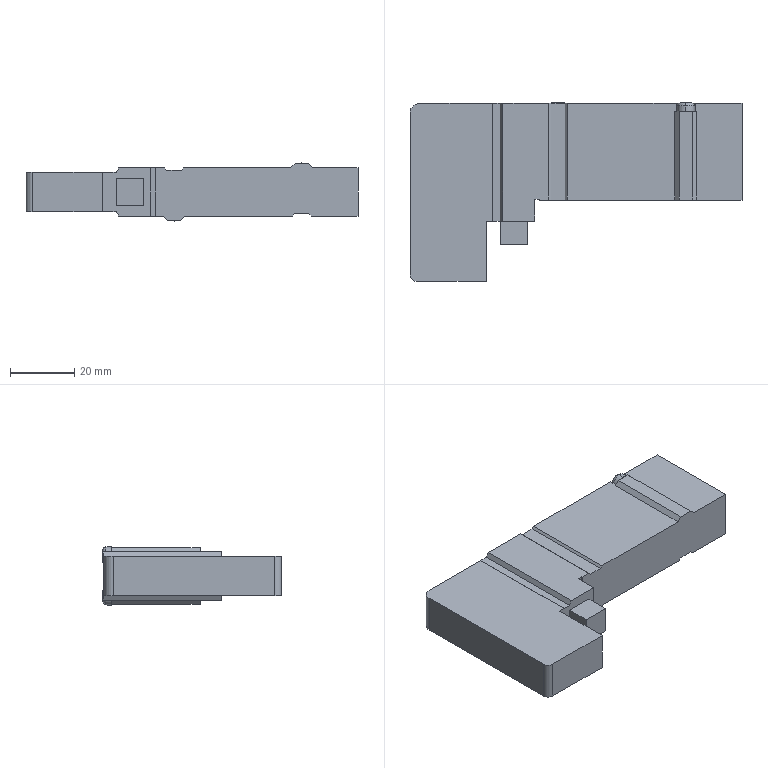Part | SolidWorks | features BaseBody 1 | 1 solid | 225 faces | box 103.4 x 55.58 x 18.1 mm | volume 53626 mm3 | plane 181 | cylinder 40 | spline 4 | commonest cylinder face diameters 1.2 x6 0.8 x4 1 x4 1.5 x4 3.5 x4 5.5 x4